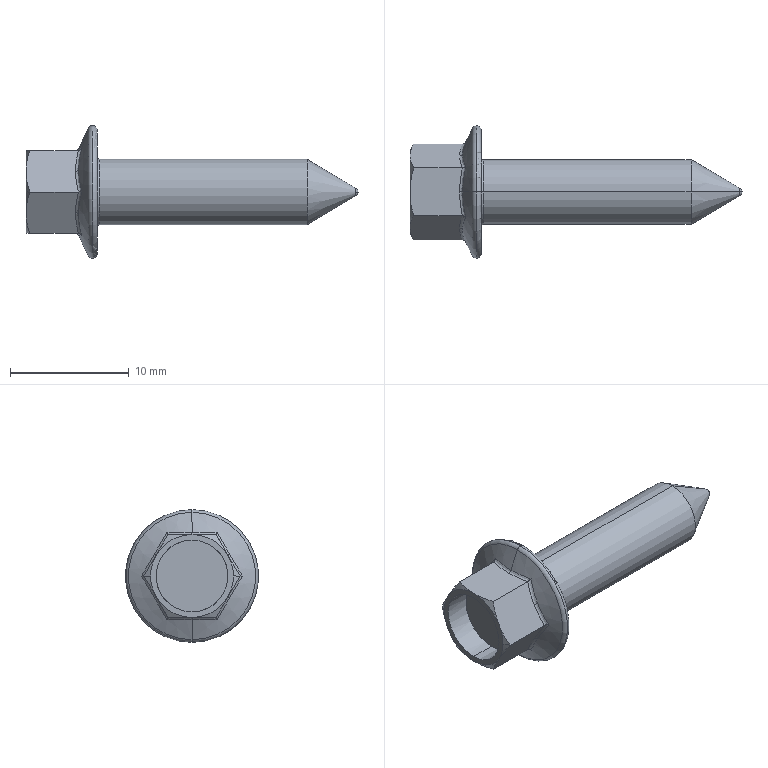Part | STEP file | 103000006194_ST5.5×22 | 1 solid | 47 faces | box 28 x 11.2 x 11.2 mm | volume 709.482 mm3 | cone 12 | spline 12 | plane 9 | torus 6 | cylinder 4 | sphere 4 | commonest cylinder face diameters 5.5 x2 6.062 x2